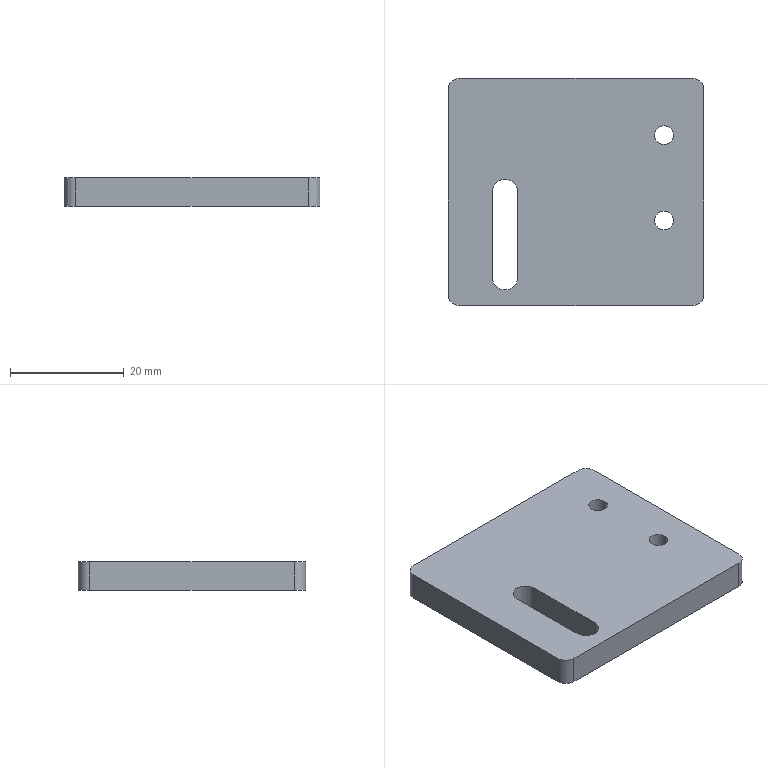Part | STEP file | H_ND24021-JJ-05-02B-BJ | 1 solid | 18 faces | box 45 x 40 x 5 mm | volume 8480 mm3 | cylinder 10 | plane 8 | commonest cylinder face diameters 3.3 x4 4 x4 4.5 x2